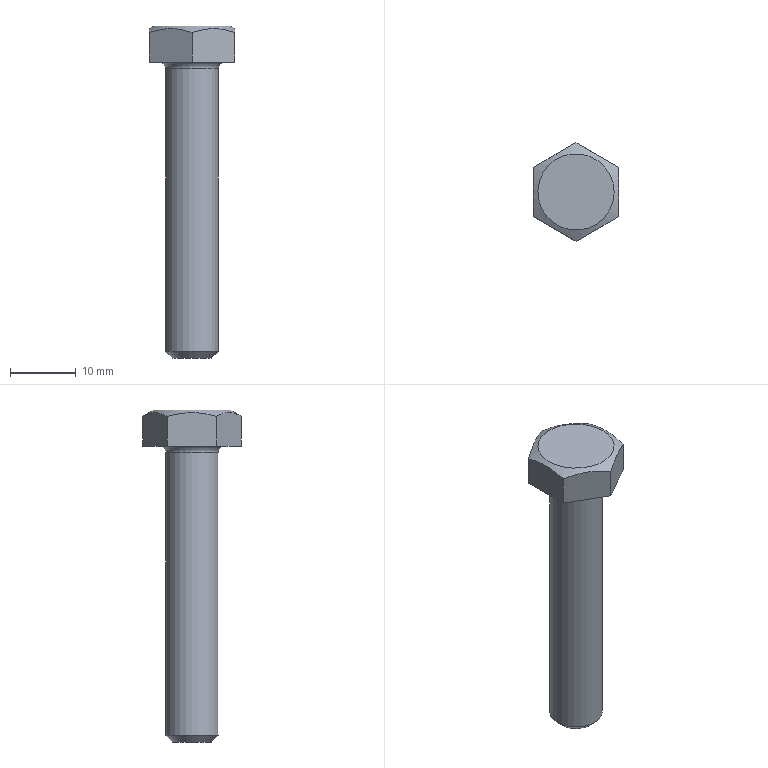Part | STEP file | SI10845 | 1 solid | 13 faces | box 13 x 15.011 x 50.5 mm | volume 3048 mm3 | plane 9 | cone 2 | cylinder 1 | torus 1 | commonest cylinder face diameters 8 x1
STEP:
#1=CARTESIAN_POINT('',(-5.,0.,0.));
#2=VERTEX_POINT('',#1);
#3=CARTESIAN_POINT('',(0.,0.,0.));
#4=DIRECTION('',(0.,0.,1.));
#5=DIRECTION('',(-1.,0.,0.));
#6=AXIS2_PLACEMENT_3D('',#3,#4,#5);
#7=CIRCLE('',#6,5.);
#8=EDGE_CURVE('',#2,#2,#7,.T.);
#9=ORIENTED_EDGE('',*,*,#8,.T.);
#10=EDGE_LOOP('',(#9));
#11=FACE_BOUND('',#10,.T.);
#12=CARTESIAN_POINT('',(6.5,3.753,0.));
#13=VERTEX_POINT('',#12);
#14=CARTESIAN_POINT('',(0.,7.506,0.));
#15=VERTEX_POINT('',#14);
#16=CARTESIAN_POINT('',(6.5,3.753,0.));
#17=DIRECTION('',(-0.866,0.5,0.));
#18=VECTOR('',#17,1000.);
#19=LINE('',#16,#18);
#20=EDGE_CURVE('',#13,#15,#19,.T.);
#21=ORIENTED_EDGE('',*,*,#20,.F.);
#22=CARTESIAN_POINT('',(6.5,-3.753,0.));
#23=VERTEX_POINT('',#22);
#24=CARTESIAN_POINT('',(6.5,-3.753,0.));
#25=DIRECTION('',(0.,1.,0.));
#26=VECTOR('',#25,1000.);
#27=LINE('',#24,#26);
#28=EDGE_CURVE('',#23,#13,#27,.T.);
#29=ORIENTED_EDGE('',*,*,#28,.F.);
#30=CARTESIAN_POINT('',(0.,-7.506,0.));
#31=VERTEX_POINT('',#30);
#32=CARTESIAN_POINT('',(0.,-7.506,0.));
#33=DIRECTION('',(0.866,0.5,0.));
#34=VECTOR('',#33,1000.);
#35=LINE('',#32,#34);
#36=EDGE_CURVE('',#31,#23,#35,.T.);
#37=ORIENTED_EDGE('',*,*,#36,.F.);
#38=CARTESIAN_POINT('',(-6.5,-3.753,0.));
#39=VERTEX_POINT('',#38);
#40=CARTESIAN_POINT('',(-6.5,-3.753,0.));
#41=DIRECTION('',(0.866,-0.5,0.));
#42=VECTOR('',#41,1000.);
#43=LINE('',#40,#42);
#44=EDGE_CURVE('',#39,#31,#43,.T.);
#45=ORIENTED_EDGE('',*,*,#44,.F.);
#46=CARTESIAN_POINT('',(-6.5,3.753,0.));
#47=VERTEX_POINT('',#46);
#48=CARTESIAN_POINT('',(-6.5,3.753,0.));
#49=DIRECTION('',(0.,-1.,0.));
#50=VECTOR('',#49,1000.);
#51=LINE('',#48,#50);
#52=EDGE_CURVE('',#47,#39,#51,.T.);
#53=ORIENTED_EDGE('',*,*,#52,.F.);
#54=CARTESIAN_POINT('',(0.,7.506,0.));
#55=DIRECTION('',(-0.866,-0.5,0.));
#56=VECTOR('',#55,1000.);
#57=LINE('',#54,#56);
#58=EDGE_CURVE('',#15,#47,#57,.T.);
#59=ORIENTED_EDGE('',*,*,#58,.F.);
#60=EDGE_LOOP('',(#21,#29,#37,#45,#53,#59));
#61=FACE_OUTER_BOUND('',#60,.T.);
#62=CARTESIAN_POINT('',(6.5,3.753,0.));
#63=DIRECTION('',(0.,0.,-1.));
#64=DIRECTION('',(-1.,0.,0.));
#65=AXIS2_PLACEMENT_3D('',#62,#63,#64);
#66=PLANE('',#65);
#67=ADVANCED_FACE('',(#11,#61),#66,.T.);
#68=CARTESIAN_POINT('',(6.5,3.753,4.515));
#69=VERTEX_POINT('',#68);
#70=CARTESIAN_POINT('',(0.,7.506,4.515));
#71=VERTEX_POINT('',#70);
#72=CARTESIAN_POINT('',(6.5,3.753,4.515));
#73=CARTESIAN_POINT('',(5.969,4.059,4.692));
#74=CARTESIAN_POINT('',(5.435,4.368,4.838));
#75=CARTESIAN_POINT('',(4.355,4.991,5.04));
#76=CARTESIAN_POINT('',(3.809,5.307,5.095));
#77=CARTESIAN_POINT('',(2.98,5.785,5.096));
#78=CARTESIAN_POINT('',(2.702,5.945,5.082));
#79=CARTESIAN_POINT('',(2.153,6.262,5.03));
#80=CARTESIAN_POINT('',(1.88,6.42,4.99));
#81=CARTESIAN_POINT('',(1.067,6.889,4.839));
#82=CARTESIAN_POINT('',(0.5313,7.199,4.692));
#83=CARTESIAN_POINT('',(0.,7.506,4.515));
#84=B_SPLINE_CURVE_WITH_KNOTS('',3,(#72,#73,#74,#75,#76,#77,#78,#79,#80,#81,#82,#83),.UNSPECIFIED.,.F.,.F.,(4,2,2,2,2,4),(0.000000238,0.001895,0.00379,0.004738,0.005685,0.00758),.UNSPECIFIED.);
#85=EDGE_CURVE('',#69,#71,#84,.T.);
#86=ORIENTED_EDGE('',*,*,#85,.F.);
#87=CARTESIAN_POINT('',(6.5,3.753,5.5));
#88=DIRECTION('',(0.,0.,-1.));
#89=VECTOR('',#88,1000.);
#90=LINE('',#87,#89);
#91=EDGE_CURVE('',#69,#13,#90,.T.);
#92=ORIENTED_EDGE('',*,*,#91,.T.);
#93=ORIENTED_EDGE('',*,*,#20,.T.);
#94=CARTESIAN_POINT('',(0.,7.506,5.5));
#95=DIRECTION('',(0.,0.,-1.));
#96=VECTOR('',#95,1000.);
#97=LINE('',#94,#96);
#98=EDGE_CURVE('',#71,#15,#97,.T.);
#99=ORIENTED_EDGE('',*,*,#98,.F.);
#100=EDGE_LOOP('',(#86,#92,#93,#99));
#101=FACE_OUTER_BOUND('',#100,.T.);
#102=CARTESIAN_POINT('',(6.5,3.753,5.5));
#103=DIRECTION('',(-0.5,-0.866,0.));
#104=DIRECTION('',(0.866,-0.5,0.));
#105=AXIS2_PLACEMENT_3D('',#102,#103,#104);
#106=PLANE('',#105);
#107=ADVANCED_FACE('',(#101),#106,.F.);
#108=CARTESIAN_POINT('',(-6.5,3.753,4.515));
#109=VERTEX_POINT('',#108);
#110=CARTESIAN_POINT('',(0.,7.506,4.515));
#111=CARTESIAN_POINT('',(-0.5307,7.199,4.692));
#112=CARTESIAN_POINT('',(-1.065,6.891,4.838));
#113=CARTESIAN_POINT('',(-2.145,6.267,5.04));
#114=CARTESIAN_POINT('',(-2.691,5.952,5.095));
#115=CARTESIAN_POINT('',(-3.52,5.473,5.096));
#116=CARTESIAN_POINT('',(-3.798,5.313,5.082));
#117=CARTESIAN_POINT('',(-4.347,4.996,5.03));
#118=CARTESIAN_POINT('',(-4.62,4.838,4.99));
#119=CARTESIAN_POINT('',(-5.433,4.369,4.839));
#120=CARTESIAN_POINT('',(-5.969,4.06,4.692));
#121=CARTESIAN_POINT('',(-6.5,3.753,4.515));
#122=B_SPLINE_CURVE_WITH_KNOTS('',3,(#110,#111,#112,#113,#114,#115,#116,#117,#118,#119,#120,#121),.UNSPECIFIED.,.F.,.F.,(4,2,2,2,2,4),(0.000000238,0.001895,0.00379,0.004738,0.005685,0.00758),.UNSPECIFIED.);
#123=EDGE_CURVE('',#71,#109,#122,.T.);
#124=ORIENTED_EDGE('',*,*,#123,.F.);
#125=ORIENTED_EDGE('',*,*,#98,.T.);
#126=ORIENTED_EDGE('',*,*,#58,.T.);
#127=CARTESIAN_POINT('',(-6.5,3.753,5.5));
#128=DIRECTION('',(0.,0.,-1.));
#129=VECTOR('',#128,1000.);
#130=LINE('',#127,#129);
#131=EDGE_CURVE('',#109,#47,#130,.T.);
#132=ORIENTED_EDGE('',*,*,#131,.F.);
#133=EDGE_LOOP('',(#124,#125,#126,#132));
#134=FACE_OUTER_BOUND('',#133,.T.);
#135=CARTESIAN_POINT('',(0.,7.506,5.5));
#136=DIRECTION('',(0.5,-0.866,0.));
#137=DIRECTION('',(0.866,0.5,0.));
#138=AXIS2_PLACEMENT_3D('',#135,#136,#137);
#139=PLANE('',#138);
#140=ADVANCED_FACE('',(#134),#139,.F.);
#141=CARTESIAN_POINT('',(-6.5,-3.753,4.515));
#142=VERTEX_POINT('',#141);
#143=CARTESIAN_POINT('',(-6.5,3.753,4.515));
#144=CARTESIAN_POINT('',(-6.5,3.146,4.69));
#145=CARTESIAN_POINT('',(-6.5,2.532,4.836));
#146=CARTESIAN_POINT('',(-6.5,1.279,5.04));
#147=CARTESIAN_POINT('',(-6.5,0.6357,5.096));
#148=CARTESIAN_POINT('',(-6.5,-0.6333,5.096));
#149=CARTESIAN_POINT('',(-6.5,-1.264,5.041));
#150=CARTESIAN_POINT('',(-6.5,-2.517,4.839));
#151=CARTESIAN_POINT('',(-6.5,-3.142,4.692));
#152=CARTESIAN_POINT('',(-6.5,-3.753,4.515));
#153=B_SPLINE_CURVE_WITH_KNOTS('',3,(#143,#144,#145,#146,#147,#148,#149,#150,#151,#152),.UNSPECIFIED.,.F.,.F.,(4,2,2,2,4),(0.01728,0.01918,0.02109,0.02299,0.02489),.UNSPECIFIED.);
#154=EDGE_CURVE('',#109,#142,#153,.T.);
#155=ORIENTED_EDGE('',*,*,#154,.F.);
#156=ORIENTED_EDGE('',*,*,#131,.T.);
#157=ORIENTED_EDGE('',*,*,#52,.T.);
#158=CARTESIAN_POINT('',(-6.5,-3.753,5.5));
#159=DIRECTION('',(0.,0.,-1.));
#160=VECTOR('',#159,1000.);
#161=LINE('',#158,#160);
#162=EDGE_CURVE('',#142,#39,#161,.T.);
#163=ORIENTED_EDGE('',*,*,#162,.F.);
#164=EDGE_LOOP('',(#155,#156,#157,#163));
#165=FACE_OUTER_BOUND('',#164,.T.);
#166=CARTESIAN_POINT('',(-6.5,3.753,5.5));
#167=DIRECTION('',(1.,0.,0.));
#168=DIRECTION('',(0.,0.,-1.));
#169=AXIS2_PLACEMENT_3D('',#166,#167,#168);
#170=PLANE('',#169);
#171=ADVANCED_FACE('',(#165),#170,.F.);
#172=CARTESIAN_POINT('',(0.,-7.506,4.515));
#173=VERTEX_POINT('',#172);
#174=CARTESIAN_POINT('',(-6.5,-3.753,4.515));
#175=CARTESIAN_POINT('',(-5.969,-4.059,4.692));
#176=CARTESIAN_POINT('',(-5.435,-4.368,4.838));
#177=CARTESIAN_POINT('',(-4.355,-4.991,5.04));
#178=CARTESIAN_POINT('',(-3.809,-5.307,5.095));
#179=CARTESIAN_POINT('',(-2.98,-5.785,5.096));
#180=CARTESIAN_POINT('',(-2.702,-5.945,5.082));
#181=CARTESIAN_POINT('',(-2.153,-6.262,5.03));
#182=CARTESIAN_POINT('',(-1.88,-6.42,4.99));
#183=CARTESIAN_POINT('',(-1.067,-6.889,4.839));
#184=CARTESIAN_POINT('',(-0.5313,-7.199,4.692));
#185=CARTESIAN_POINT('',(0.,-7.506,4.515));
#186=B_SPLINE_CURVE_WITH_KNOTS('',3,(#174,#175,#176,#177,#178,#179,#180,#181,#182,#183,#184,#185),.UNSPECIFIED.,.F.,.F.,(4,2,2,2,2,4),(0.000000238,0.001895,0.00379,0.004738,0.005685,0.00758),.UNSPECIFIED.);
#187=EDGE_CURVE('',#142,#173,#186,.T.);
#188=ORIENTED_EDGE('',*,*,#187,.F.);
#189=ORIENTED_EDGE('',*,*,#162,.T.);
#190=ORIENTED_EDGE('',*,*,#44,.T.);
#191=CARTESIAN_POINT('',(0.,-7.506,5.5));
#192=DIRECTION('',(0.,0.,-1.));
#193=VECTOR('',#192,1000.);
#194=LINE('',#191,#193);
#195=EDGE_CURVE('',#173,#31,#194,.T.);
#196=ORIENTED_EDGE('',*,*,#195,.F.);
#197=EDGE_LOOP('',(#188,#189,#190,#196));
#198=FACE_OUTER_BOUND('',#197,.T.);
#199=CARTESIAN_POINT('',(-6.5,-3.753,5.5));
#200=DIRECTION('',(0.5,0.866,0.));
#201=DIRECTION('',(-0.866,0.5,0.));
#202=AXIS2_PLACEMENT_3D('',#199,#200,#201);
#203=PLANE('',#202);
#204=ADVANCED_FACE('',(#198),#203,.F.);
#205=CARTESIAN_POINT('',(6.5,-3.753,4.515));
#206=VERTEX_POINT('',#205);
#207=CARTESIAN_POINT('',(0.,-7.506,4.515));
#208=CARTESIAN_POINT('',(0.5307,-7.199,4.692));
#209=CARTESIAN_POINT('',(1.065,-6.891,4.838));
#210=CARTESIAN_POINT('',(2.145,-6.267,5.04));
#211=CARTESIAN_POINT('',(2.691,-5.952,5.095));
#212=CARTESIAN_POINT('',(3.52,-5.473,5.096));
#213=CARTESIAN_POINT('',(3.798,-5.313,5.082));
#214=CARTESIAN_POINT('',(4.347,-4.996,5.03));
#215=CARTESIAN_POINT('',(4.62,-4.838,4.99));
#216=CARTESIAN_POINT('',(5.433,-4.369,4.839));
#217=CARTESIAN_POINT('',(5.969,-4.06,4.692));
#218=CARTESIAN_POINT('',(6.5,-3.753,4.515));
#219=B_SPLINE_CURVE_WITH_KNOTS('',3,(#207,#208,#209,#210,#211,#212,#213,#214,#215,#216,#217,#218),.UNSPECIFIED.,.F.,.F.,(4,2,2,2,2,4),(0.000000238,0.001895,0.00379,0.004738,0.005685,0.00758),.UNSPECIFIED.);
#220=EDGE_CURVE('',#173,#206,#219,.T.);
#221=ORIENTED_EDGE('',*,*,#220,.F.);
#222=ORIENTED_EDGE('',*,*,#195,.T.);
#223=ORIENTED_EDGE('',*,*,#36,.T.);
#224=CARTESIAN_POINT('',(6.5,-3.753,5.5));
#225=DIRECTION('',(0.,0.,-1.));
#226=VECTOR('',#225,1000.);
#227=LINE('',#224,#226);
#228=EDGE_CURVE('',#206,#23,#227,.T.);
#229=ORIENTED_EDGE('',*,*,#228,.F.);
#230=EDGE_LOOP('',(#221,#222,#223,#229));
#231=FACE_OUTER_BOUND('',#230,.T.);
#232=CARTESIAN_POINT('',(0.,-7.506,5.5));
#233=DIRECTION('',(-0.5,0.866,0.));
#234=DIRECTION('',(-0.866,-0.5,0.));
#235=AXIS2_PLACEMENT_3D('',#232,#233,#234);
#236=PLANE('',#235);
#237=ADVANCED_FACE('',(#231),#236,.F.);
#238=CARTESIAN_POINT('',(6.5,-3.753,4.515));
#239=CARTESIAN_POINT('',(6.5,-3.142,4.692));
#240=CARTESIAN_POINT('',(6.5,-2.517,4.839));
#241=CARTESIAN_POINT('',(6.5,-1.264,5.041));
#242=CARTESIAN_POINT('',(6.5,-0.6333,5.096));
#243=CARTESIAN_POINT('',(6.5,0.6357,5.096));
#244=CARTESIAN_POINT('',(6.5,1.279,5.04));
#245=CARTESIAN_POINT('',(6.5,2.532,4.836));
#246=CARTESIAN_POINT('',(6.5,3.146,4.69));
#247=CARTESIAN_POINT('',(6.5,3.753,4.515));
#248=B_SPLINE_CURVE_WITH_KNOTS('',3,(#238,#239,#240,#241,#242,#243,#244,#245,#246,#247),.UNSPECIFIED.,.F.,.F.,(4,2,2,2,4),(0.006757,0.008656,0.01056,0.01245,0.01435),.UNSPECIFIED.);
#249=EDGE_CURVE('',#206,#69,#248,.T.);
#250=ORIENTED_EDGE('',*,*,#249,.F.);
#251=ORIENTED_EDGE('',*,*,#228,.T.);
#252=ORIENTED_EDGE('',*,*,#28,.T.);
#253=ORIENTED_EDGE('',*,*,#91,.F.);
#254=EDGE_LOOP('',(#250,#251,#252,#253));
#255=FACE_OUTER_BOUND('',#254,.T.);
#256=CARTESIAN_POINT('',(6.5,-3.753,5.5));
#257=DIRECTION('',(-1.,0.,0.));
#258=DIRECTION('',(0.,-1.,0.));
#259=AXIS2_PLACEMENT_3D('',#256,#257,#258);
#260=PLANE('',#259);
#261=ADVANCED_FACE('',(#255),#260,.F.);
#262=CARTESIAN_POINT('',(5.8,0.,5.5));
#263=VERTEX_POINT('',#262);
#264=CARTESIAN_POINT('',(0.,0.,5.5));
#265=DIRECTION('',(0.,0.,1.));
#266=DIRECTION('',(1.,0.,0.));
#267=AXIS2_PLACEMENT_3D('',#264,#265,#266);
#268=CIRCLE('',#267,5.8);
#269=EDGE_CURVE('',#263,#263,#268,.T.);
#270=ORIENTED_EDGE('',*,*,#269,.F.);
#271=EDGE_LOOP('',(#270));
#272=FACE_BOUND('',#271,.T.);
#273=ORIENTED_EDGE('',*,*,#85,.T.);
#274=ORIENTED_EDGE('',*,*,#123,.T.);
#275=ORIENTED_EDGE('',*,*,#154,.T.);
#276=ORIENTED_EDGE('',*,*,#187,.T.);
#277=ORIENTED_EDGE('',*,*,#220,.T.);
#278=ORIENTED_EDGE('',*,*,#249,.T.);
#279=EDGE_LOOP('',(#273,#274,#275,#276,#277,#278));
#280=FACE_OUTER_BOUND('',#279,.T.);
#281=CARTESIAN_POINT('',(0.,0.,5.5));
#282=DIRECTION('',(0.,0.,-1.));
#283=DIRECTION('',(-1.,0.,0.));
#284=AXIS2_PLACEMENT_3D('',#281,#282,#283);
#285=CONICAL_SURFACE('',#284,5.8,1.047);
#286=ADVANCED_FACE('',(#272,#280),#285,.T.);
#287=ORIENTED_EDGE('',*,*,#269,.T.);
#288=EDGE_LOOP('',(#287));
#289=FACE_OUTER_BOUND('',#288,.T.);
#290=CARTESIAN_POINT('',(6.5,3.753,5.5));
#291=DIRECTION('',(0.,0.,-1.));
#292=DIRECTION('',(-1.,0.,0.));
#293=AXIS2_PLACEMENT_3D('',#290,#291,#292);
#294=PLANE('',#293);
#295=ADVANCED_FACE('',(#289),#294,.F.);
#296=CARTESIAN_POINT('',(-4.,0.,-1.));
#297=VERTEX_POINT('',#296);
#298=CARTESIAN_POINT('',(0.,0.,-1.));
#299=DIRECTION('',(0.,0.,-1.));
#300=DIRECTION('',(-1.,0.,0.));
#301=AXIS2_PLACEMENT_3D('',#298,#299,#300);
#302=CIRCLE('',#301,4.);
#303=EDGE_CURVE('',#297,#297,#302,.T.);
#304=ORIENTED_EDGE('',*,*,#303,.T.);
#305=EDGE_LOOP('',(#304));
#306=FACE_OUTER_BOUND('',#305,.T.);
#307=CARTESIAN_POINT('',(-4.,0.,-44.));
#308=VERTEX_POINT('',#307);
#309=CARTESIAN_POINT('',(0.,0.,-44.));
#310=DIRECTION('',(0.,0.,1.));
#311=DIRECTION('',(-1.,0.,0.));
#312=AXIS2_PLACEMENT_3D('',#309,#310,#311);
#313=CIRCLE('',#312,4.);
#314=EDGE_CURVE('',#308,#308,#313,.T.);
#315=ORIENTED_EDGE('',*,*,#314,.T.);
#316=EDGE_LOOP('',(#315));
#317=FACE_OUTER_BOUND('',#316,.T.);
#318=CARTESIAN_POINT('',(0.,0.,-45.));
#319=DIRECTION('',(0.,0.,1.));
#320=DIRECTION('',(1.,0.,0.));
#321=AXIS2_PLACEMENT_3D('',#318,#319,#320);
#322=CYLINDRICAL_SURFACE('',#321,4.);
#323=ADVANCED_FACE('',(#306,#317),#322,.T.);
#324=CARTESIAN_POINT('',(-3.,0.,-45.));
#325=VERTEX_POINT('',#324);
#326=CARTESIAN_POINT('',(0.,0.,-45.));
#327=DIRECTION('',(0.,0.,-1.));
#328=DIRECTION('',(-1.,0.,0.));
#329=AXIS2_PLACEMENT_3D('',#326,#327,#328);
#330=CIRCLE('',#329,3.);
#331=EDGE_CURVE('',#325,#325,#330,.T.);
#332=ORIENTED_EDGE('',*,*,#331,.T.);
#333=EDGE_LOOP('',(#332));
#334=FACE_OUTER_BOUND('',#333,.T.);
#335=CARTESIAN_POINT('',(0.,0.,-45.));
#336=DIRECTION('',(0.,0.,-1.));
#337=DIRECTION('',(-1.,0.,0.));
#338=AXIS2_PLACEMENT_3D('',#335,#336,#337);
#339=PLANE('',#338);
#340=ADVANCED_FACE('',(#334),#339,.T.);
#341=ORIENTED_EDGE('',*,*,#314,.F.);
#342=EDGE_LOOP('',(#341));
#343=FACE_OUTER_BOUND('',#342,.T.);
#344=ORIENTED_EDGE('',*,*,#331,.F.);
#345=EDGE_LOOP('',(#344));
#346=FACE_BOUND('',#345,.T.);
#347=CARTESIAN_POINT('',(0.,0.,-45.));
#348=DIRECTION('',(0.,0.,1.));
#349=DIRECTION('',(1.,0.,0.));
#350=AXIS2_PLACEMENT_3D('',#347,#348,#349);
#351=CONICAL_SURFACE('',#350,3.,0.7854);
#352=ADVANCED_FACE('',(#343,#346),#351,.T.);
#353=ORIENTED_EDGE('',*,*,#8,.F.);
#354=EDGE_LOOP('',(#353));
#355=FACE_OUTER_BOUND('',#354,.T.);
#356=ORIENTED_EDGE('',*,*,#303,.F.);
#357=EDGE_LOOP('',(#356));
#358=FACE_OUTER_BOUND('',#357,.T.);
#359=CARTESIAN_POINT('',(0.,0.,-1.));
#360=DIRECTION('',(0.,0.,-1.));
#361=DIRECTION('',(-1.,0.,0.));
#362=AXIS2_PLACEMENT_3D('',#359,#360,#361);
#363=TOROIDAL_SURFACE('',#362,5.,1.);
#364=ADVANCED_FACE('',(#355,#358),#363,.F.);
#365=CLOSED_SHELL('',(#67,#107,#140,#171,#204,#237,#261,#286,#295,#323,#340,#352,#364));
#366=MANIFOLD_SOLID_BREP('',#365);
#367=CARTESIAN_POINT('',(0.,0.,0.));
#368=DIRECTION('',(0.,0.,1.));
#369=DIRECTION('',(1.,0.,0.));
#370=AXIS2_PLACEMENT_3D('',#367,#368,#369);
#371=(LENGTH_UNIT()NAMED_UNIT(*)SI_UNIT(.MILLI.,.METRE.));
#372=UNCERTAINTY_MEASURE_WITH_UNIT(LENGTH_MEASURE(0.00001),#371,'','');
#373=(NAMED_UNIT(*)PLANE_ANGLE_UNIT()SI_UNIT($,.RADIAN.));
#374=(NAMED_UNIT(*)SI_UNIT($,.STERADIAN.)SOLID_ANGLE_UNIT());
#375=(GEOMETRIC_REPRESENTATION_CONTEXT(3)GLOBAL_UNCERTAINTY_ASSIGNED_CONTEXT((#372))GLOBAL_UNIT_ASSIGNED_CONTEXT((#371,#373,#374))REPRESENTATION_CONTEXT('',''));
#376=ADVANCED_BREP_SHAPE_REPRESENTATION('',(#366,#370),#375);